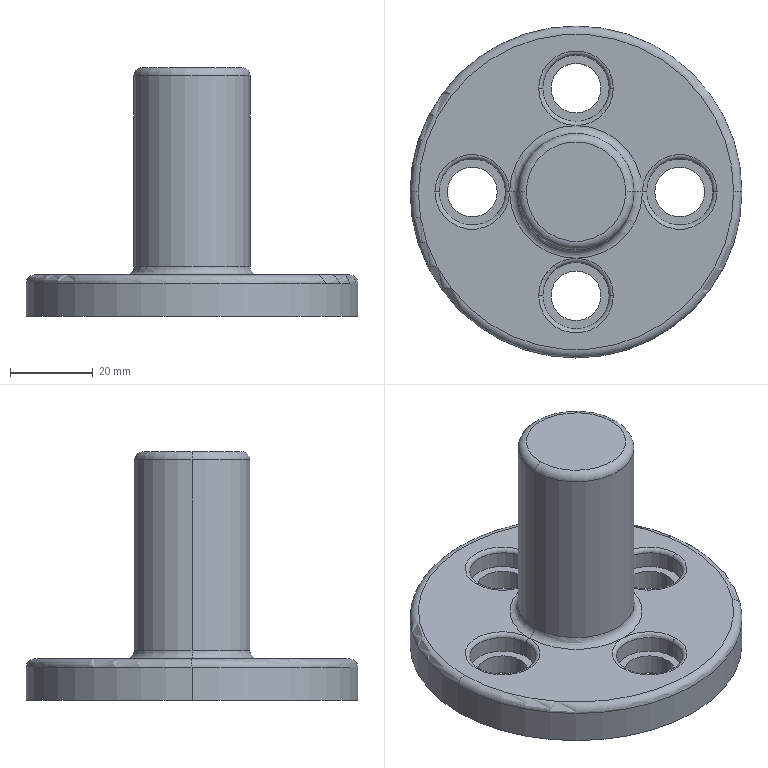Part | SolidWorks | features Fillet 4, ICE 3, Extrusion 1 | 1 solid | 41 faces | box 80 x 80 x 60 mm | volume 74517 mm3 | cylinder 20 | torus 14 | plane 7 | commonest cylinder face diameters 12 x8 16 x8 28 x2 80 x2
STEP:
#1=CARTESIAN_POINT('',(-14.,0.,12.));
#2=VERTEX_POINT('',#1);
#3=CARTESIAN_POINT('',(14.,0.,12.));
#4=VERTEX_POINT('',#3);
#5=CARTESIAN_POINT('',(0.,0.,12.));
#6=DIRECTION('',(0.,0.,1.));
#7=DIRECTION('',(1.,0.,0.));
#8=AXIS2_PLACEMENT_3D('',#5,#6,#7);
#9=CIRCLE('',#8,14.);
#10=EDGE_CURVE('',#2,#4,#9,.T.);
#11=ORIENTED_EDGE('',*,*,#10,.F.);
#12=CARTESIAN_POINT('',(-16.,0.,10.));
#13=VERTEX_POINT('',#12);
#14=CARTESIAN_POINT('',(-16.,0.,12.));
#15=DIRECTION('',(0.,1.,0.));
#16=DIRECTION('',(-1.,0.,0.));
#17=AXIS2_PLACEMENT_3D('',#14,#15,#16);
#18=CIRCLE('',#17,2.);
#19=EDGE_CURVE('',#2,#13,#18,.T.);
#20=ORIENTED_EDGE('',*,*,#19,.T.);
#21=CARTESIAN_POINT('',(0.,-16.,10.));
#22=VERTEX_POINT('',#21);
#23=CARTESIAN_POINT('',(0.,0.,10.));
#24=DIRECTION('',(0.,0.,-1.));
#25=DIRECTION('',(1.,0.,0.));
#26=AXIS2_PLACEMENT_3D('',#23,#24,#25);
#27=CIRCLE('',#26,16.);
#28=EDGE_CURVE('',#22,#13,#27,.T.);
#29=ORIENTED_EDGE('',*,*,#28,.F.);
#30=CARTESIAN_POINT('',(16.,0.,10.));
#31=VERTEX_POINT('',#30);
#32=CARTESIAN_POINT('',(0.,0.,10.));
#33=DIRECTION('',(0.,0.,-1.));
#34=DIRECTION('',(1.,0.,0.));
#35=AXIS2_PLACEMENT_3D('',#32,#33,#34);
#36=CIRCLE('',#35,16.);
#37=EDGE_CURVE('',#31,#22,#36,.T.);
#38=ORIENTED_EDGE('',*,*,#37,.F.);
#39=CARTESIAN_POINT('',(16.,0.,12.));
#40=DIRECTION('',(0.,-1.,0.));
#41=DIRECTION('',(0.,0.,-1.));
#42=AXIS2_PLACEMENT_3D('',#39,#40,#41);
#43=CIRCLE('',#42,2.);
#44=EDGE_CURVE('',#4,#31,#43,.T.);
#45=ORIENTED_EDGE('',*,*,#44,.F.);
#46=EDGE_LOOP('',(#11,#20,#29,#38,#45));
#47=FACE_OUTER_BOUND('',#46,.T.);
#48=CARTESIAN_POINT('',(0.,0.,12.));
#49=DIRECTION('',(0.,0.,1.));
#50=DIRECTION('',(1.,0.,0.));
#51=AXIS2_PLACEMENT_3D('',#48,#49,#50);
#52=TOROIDAL_SURFACE('',#51,16.,2.);
#53=ADVANCED_FACE('',(#47),#52,.F.);
#54=CARTESIAN_POINT('',(-14.,0.,58.));
#55=VERTEX_POINT('',#54);
#56=CARTESIAN_POINT('',(14.,0.,58.));
#57=VERTEX_POINT('',#56);
#58=CARTESIAN_POINT('',(0.,0.,58.));
#59=DIRECTION('',(0.,0.,-1.));
#60=DIRECTION('',(1.,0.,0.));
#61=AXIS2_PLACEMENT_3D('',#58,#59,#60);
#62=CIRCLE('',#61,14.);
#63=EDGE_CURVE('',#55,#57,#62,.T.);
#64=ORIENTED_EDGE('',*,*,#63,.F.);
#65=CARTESIAN_POINT('',(-12.,0.,60.));
#66=VERTEX_POINT('',#65);
#67=CARTESIAN_POINT('',(-12.,0.,58.));
#68=DIRECTION('',(0.,1.,0.));
#69=DIRECTION('',(-1.,0.,0.));
#70=AXIS2_PLACEMENT_3D('',#67,#68,#69);
#71=CIRCLE('',#70,2.);
#72=EDGE_CURVE('',#55,#66,#71,.T.);
#73=ORIENTED_EDGE('',*,*,#72,.T.);
#74=CARTESIAN_POINT('',(12.,0.,60.));
#75=VERTEX_POINT('',#74);
#76=CARTESIAN_POINT('',(0.,0.,60.));
#77=DIRECTION('',(0.,0.,1.));
#78=DIRECTION('',(1.,0.,0.));
#79=AXIS2_PLACEMENT_3D('',#76,#77,#78);
#80=CIRCLE('',#79,12.);
#81=EDGE_CURVE('',#75,#66,#80,.T.);
#82=ORIENTED_EDGE('',*,*,#81,.F.);
#83=CARTESIAN_POINT('',(12.,0.,58.));
#84=DIRECTION('',(0.,-1.,0.));
#85=DIRECTION('',(0.,0.,-1.));
#86=AXIS2_PLACEMENT_3D('',#83,#84,#85);
#87=CIRCLE('',#86,2.);
#88=EDGE_CURVE('',#57,#75,#87,.T.);
#89=ORIENTED_EDGE('',*,*,#88,.F.);
#90=EDGE_LOOP('',(#64,#73,#82,#89));
#91=FACE_OUTER_BOUND('',#90,.T.);
#92=CARTESIAN_POINT('',(0.,0.,58.));
#93=DIRECTION('',(0.,0.,1.));
#94=DIRECTION('',(1.,0.,0.));
#95=AXIS2_PLACEMENT_3D('',#92,#93,#94);
#96=TOROIDAL_SURFACE('',#95,12.,2.);
#97=ADVANCED_FACE('',(#91),#96,.T.);
#98=ORIENTED_EDGE('',*,*,#63,.T.);
#99=CARTESIAN_POINT('',(14.,0.,60.));
#100=DIRECTION('',(0.,0.,-1.));
#101=VECTOR('',#100,1000.);
#102=LINE('',#99,#101);
#103=EDGE_CURVE('',#57,#4,#102,.T.);
#104=ORIENTED_EDGE('',*,*,#103,.T.);
#105=CARTESIAN_POINT('',(0.,0.,12.));
#106=DIRECTION('',(0.,0.,1.));
#107=DIRECTION('',(1.,0.,0.));
#108=AXIS2_PLACEMENT_3D('',#105,#106,#107);
#109=CIRCLE('',#108,14.);
#110=EDGE_CURVE('',#4,#2,#109,.T.);
#111=ORIENTED_EDGE('',*,*,#110,.T.);
#112=CARTESIAN_POINT('',(-14.,0.,60.));
#113=DIRECTION('',(0.,0.,-1.));
#114=VECTOR('',#113,1000.);
#115=LINE('',#112,#114);
#116=EDGE_CURVE('',#55,#2,#115,.T.);
#117=ORIENTED_EDGE('',*,*,#116,.F.);
#118=EDGE_LOOP('',(#98,#104,#111,#117));
#119=FACE_OUTER_BOUND('',#118,.T.);
#120=CARTESIAN_POINT('',(0.,0.,60.));
#121=DIRECTION('',(0.,0.,-1.));
#122=DIRECTION('',(-1.,0.,0.));
#123=AXIS2_PLACEMENT_3D('',#120,#121,#122);
#124=CYLINDRICAL_SURFACE('',#123,14.);
#125=ADVANCED_FACE('',(#119),#124,.T.);
#126=CARTESIAN_POINT('',(-31.,0.,0.));
#127=VERTEX_POINT('',#126);
#128=CARTESIAN_POINT('',(-19.,0.,0.));
#129=VERTEX_POINT('',#128);
#130=CARTESIAN_POINT('',(-25.,0.,0.));
#131=DIRECTION('',(0.,0.,1.));
#132=DIRECTION('',(1.,0.,0.));
#133=AXIS2_PLACEMENT_3D('',#130,#131,#132);
#134=CIRCLE('',#133,6.);
#135=EDGE_CURVE('',#127,#129,#134,.T.);
#136=ORIENTED_EDGE('',*,*,#135,.F.);
#137=CARTESIAN_POINT('',(-31.,0.,5.));
#138=VERTEX_POINT('',#137);
#139=CARTESIAN_POINT('',(-31.,0.,0.));
#140=DIRECTION('',(0.,0.,1.));
#141=VECTOR('',#140,1000.);
#142=LINE('',#139,#141);
#143=EDGE_CURVE('',#127,#138,#142,.T.);
#144=ORIENTED_EDGE('',*,*,#143,.T.);
#145=CARTESIAN_POINT('',(-19.,0.,5.));
#146=VERTEX_POINT('',#145);
#147=CARTESIAN_POINT('',(-25.,0.,5.));
#148=DIRECTION('',(0.,0.,1.));
#149=DIRECTION('',(1.,0.,0.));
#150=AXIS2_PLACEMENT_3D('',#147,#148,#149);
#151=CIRCLE('',#150,6.);
#152=EDGE_CURVE('',#138,#146,#151,.T.);
#153=ORIENTED_EDGE('',*,*,#152,.T.);
#154=CARTESIAN_POINT('',(-19.,0.,0.));
#155=DIRECTION('',(0.,0.,1.));
#156=VECTOR('',#155,1000.);
#157=LINE('',#154,#156);
#158=EDGE_CURVE('',#129,#146,#157,.T.);
#159=ORIENTED_EDGE('',*,*,#158,.F.);
#160=EDGE_LOOP('',(#136,#144,#153,#159));
#161=FACE_OUTER_BOUND('',#160,.T.);
#162=CARTESIAN_POINT('',(-25.,0.,0.));
#163=DIRECTION('',(0.,0.,1.));
#164=DIRECTION('',(1.,0.,0.));
#165=AXIS2_PLACEMENT_3D('',#162,#163,#164);
#166=CYLINDRICAL_SURFACE('',#165,6.);
#167=ADVANCED_FACE('',(#161),#166,.F.);
#168=CARTESIAN_POINT('',(-6.,-25.,0.));
#169=VERTEX_POINT('',#168);
#170=CARTESIAN_POINT('',(6.,-25.,0.));
#171=VERTEX_POINT('',#170);
#172=CARTESIAN_POINT('',(0.,-25.,0.));
#173=DIRECTION('',(0.,0.,1.));
#174=DIRECTION('',(1.,0.,0.));
#175=AXIS2_PLACEMENT_3D('',#172,#173,#174);
#176=CIRCLE('',#175,6.);
#177=EDGE_CURVE('',#169,#171,#176,.T.);
#178=ORIENTED_EDGE('',*,*,#177,.F.);
#179=CARTESIAN_POINT('',(-6.,-25.,5.));
#180=VERTEX_POINT('',#179);
#181=CARTESIAN_POINT('',(-6.,-25.,0.));
#182=DIRECTION('',(0.,0.,1.));
#183=VECTOR('',#182,1000.);
#184=LINE('',#181,#183);
#185=EDGE_CURVE('',#169,#180,#184,.T.);
#186=ORIENTED_EDGE('',*,*,#185,.T.);
#187=CARTESIAN_POINT('',(6.,-25.,5.));
#188=VERTEX_POINT('',#187);
#189=CARTESIAN_POINT('',(0.,-25.,5.));
#190=DIRECTION('',(0.,0.,1.));
#191=DIRECTION('',(1.,0.,0.));
#192=AXIS2_PLACEMENT_3D('',#189,#190,#191);
#193=CIRCLE('',#192,6.);
#194=EDGE_CURVE('',#180,#188,#193,.T.);
#195=ORIENTED_EDGE('',*,*,#194,.T.);
#196=CARTESIAN_POINT('',(6.,-25.,0.));
#197=DIRECTION('',(0.,0.,1.));
#198=VECTOR('',#197,1000.);
#199=LINE('',#196,#198);
#200=EDGE_CURVE('',#171,#188,#199,.T.);
#201=ORIENTED_EDGE('',*,*,#200,.F.);
#202=EDGE_LOOP('',(#178,#186,#195,#201));
#203=FACE_OUTER_BOUND('',#202,.T.);
#204=CARTESIAN_POINT('',(0.,-25.,0.));
#205=DIRECTION('',(0.,0.,1.));
#206=DIRECTION('',(1.,0.,0.));
#207=AXIS2_PLACEMENT_3D('',#204,#205,#206);
#208=CYLINDRICAL_SURFACE('',#207,6.);
#209=ADVANCED_FACE('',(#203),#208,.F.);
#210=CARTESIAN_POINT('',(19.,0.,0.));
#211=VERTEX_POINT('',#210);
#212=CARTESIAN_POINT('',(31.,0.,0.));
#213=VERTEX_POINT('',#212);
#214=CARTESIAN_POINT('',(25.,0.,0.));
#215=DIRECTION('',(0.,0.,1.));
#216=DIRECTION('',(1.,0.,0.));
#217=AXIS2_PLACEMENT_3D('',#214,#215,#216);
#218=CIRCLE('',#217,6.);
#219=EDGE_CURVE('',#211,#213,#218,.T.);
#220=ORIENTED_EDGE('',*,*,#219,.F.);
#221=CARTESIAN_POINT('',(19.,0.,5.));
#222=VERTEX_POINT('',#221);
#223=CARTESIAN_POINT('',(19.,0.,0.));
#224=DIRECTION('',(0.,0.,1.));
#225=VECTOR('',#224,1000.);
#226=LINE('',#223,#225);
#227=EDGE_CURVE('',#211,#222,#226,.T.);
#228=ORIENTED_EDGE('',*,*,#227,.T.);
#229=CARTESIAN_POINT('',(31.,0.,5.));
#230=VERTEX_POINT('',#229);
#231=CARTESIAN_POINT('',(25.,0.,5.));
#232=DIRECTION('',(0.,0.,1.));
#233=DIRECTION('',(1.,0.,0.));
#234=AXIS2_PLACEMENT_3D('',#231,#232,#233);
#235=CIRCLE('',#234,6.);
#236=EDGE_CURVE('',#222,#230,#235,.T.);
#237=ORIENTED_EDGE('',*,*,#236,.T.);
#238=CARTESIAN_POINT('',(31.,0.,0.));
#239=DIRECTION('',(0.,0.,1.));
#240=VECTOR('',#239,1000.);
#241=LINE('',#238,#240);
#242=EDGE_CURVE('',#213,#230,#241,.T.);
#243=ORIENTED_EDGE('',*,*,#242,.F.);
#244=EDGE_LOOP('',(#220,#228,#237,#243));
#245=FACE_OUTER_BOUND('',#244,.T.);
#246=CARTESIAN_POINT('',(25.,0.,0.));
#247=DIRECTION('',(0.,0.,1.));
#248=DIRECTION('',(1.,0.,0.));
#249=AXIS2_PLACEMENT_3D('',#246,#247,#248);
#250=CYLINDRICAL_SURFACE('',#249,6.);
#251=ADVANCED_FACE('',(#245),#250,.F.);
#252=CARTESIAN_POINT('',(-6.,25.,0.));
#253=VERTEX_POINT('',#252);
#254=CARTESIAN_POINT('',(6.,25.,0.));
#255=VERTEX_POINT('',#254);
#256=CARTESIAN_POINT('',(0.,25.,0.));
#257=DIRECTION('',(0.,0.,1.));
#258=DIRECTION('',(1.,0.,0.));
#259=AXIS2_PLACEMENT_3D('',#256,#257,#258);
#260=CIRCLE('',#259,6.);
#261=EDGE_CURVE('',#253,#255,#260,.T.);
#262=ORIENTED_EDGE('',*,*,#261,.F.);
#263=CARTESIAN_POINT('',(-6.,25.,5.));
#264=VERTEX_POINT('',#263);
#265=CARTESIAN_POINT('',(-6.,25.,0.));
#266=DIRECTION('',(0.,0.,1.));
#267=VECTOR('',#266,1000.);
#268=LINE('',#265,#267);
#269=EDGE_CURVE('',#253,#264,#268,.T.);
#270=ORIENTED_EDGE('',*,*,#269,.T.);
#271=CARTESIAN_POINT('',(6.,25.,5.));
#272=VERTEX_POINT('',#271);
#273=CARTESIAN_POINT('',(0.,25.,5.));
#274=DIRECTION('',(0.,0.,1.));
#275=DIRECTION('',(1.,0.,0.));
#276=AXIS2_PLACEMENT_3D('',#273,#274,#275);
#277=CIRCLE('',#276,6.);
#278=EDGE_CURVE('',#264,#272,#277,.T.);
#279=ORIENTED_EDGE('',*,*,#278,.T.);
#280=CARTESIAN_POINT('',(6.,25.,0.));
#281=DIRECTION('',(0.,0.,1.));
#282=VECTOR('',#281,1000.);
#283=LINE('',#280,#282);
#284=EDGE_CURVE('',#255,#272,#283,.T.);
#285=ORIENTED_EDGE('',*,*,#284,.F.);
#286=EDGE_LOOP('',(#262,#270,#279,#285));
#287=FACE_OUTER_BOUND('',#286,.T.);
#288=CARTESIAN_POINT('',(0.,25.,0.));
#289=DIRECTION('',(0.,0.,1.));
#290=DIRECTION('',(1.,0.,0.));
#291=AXIS2_PLACEMENT_3D('',#288,#289,#290);
#292=CYLINDRICAL_SURFACE('',#291,6.);
#293=ADVANCED_FACE('',(#287),#292,.F.);
#294=CARTESIAN_POINT('',(-34.,0.,10.));
#295=VERTEX_POINT('',#294);
#296=CARTESIAN_POINT('',(-25.,0.,10.));
#297=DIRECTION('',(0.,0.,-1.));
#298=DIRECTION('',(1.,0.,0.));
#299=AXIS2_PLACEMENT_3D('',#296,#297,#298);
#300=CIRCLE('',#299,9.);
#301=EDGE_CURVE('',#295,#13,#300,.T.);
#302=ORIENTED_EDGE('',*,*,#301,.F.);
#303=CARTESIAN_POINT('',(-33.,0.,9.));
#304=VERTEX_POINT('',#303);
#305=CARTESIAN_POINT('',(-34.,0.,9.));
#306=DIRECTION('',(0.,1.,0.));
#307=DIRECTION('',(-1.,0.,0.));
#308=AXIS2_PLACEMENT_3D('',#305,#306,#307);
#309=CIRCLE('',#308,1.);
#310=EDGE_CURVE('',#295,#304,#309,.T.);
#311=ORIENTED_EDGE('',*,*,#310,.T.);
#312=CARTESIAN_POINT('',(-17.,0.,9.));
#313=VERTEX_POINT('',#312);
#314=CARTESIAN_POINT('',(-25.,0.,9.));
#315=DIRECTION('',(0.,0.,1.));
#316=DIRECTION('',(1.,0.,0.));
#317=AXIS2_PLACEMENT_3D('',#314,#315,#316);
#318=CIRCLE('',#317,8.);
#319=EDGE_CURVE('',#313,#304,#318,.T.);
#320=ORIENTED_EDGE('',*,*,#319,.F.);
#321=CARTESIAN_POINT('',(-16.,0.,9.));
#322=DIRECTION('',(0.,-1.,0.));
#323=DIRECTION('',(0.,0.,-1.));
#324=AXIS2_PLACEMENT_3D('',#321,#322,#323);
#325=CIRCLE('',#324,1.);
#326=EDGE_CURVE('',#13,#313,#325,.T.);
#327=ORIENTED_EDGE('',*,*,#326,.F.);
#328=EDGE_LOOP('',(#302,#311,#320,#327));
#329=FACE_OUTER_BOUND('',#328,.T.);
#330=CARTESIAN_POINT('',(-25.,0.,9.));
#331=DIRECTION('',(0.,0.,1.));
#332=DIRECTION('',(1.,0.,0.));
#333=AXIS2_PLACEMENT_3D('',#330,#331,#332);
#334=TOROIDAL_SURFACE('',#333,9.,1.);
#335=ADVANCED_FACE('',(#329),#334,.T.);
#336=CARTESIAN_POINT('',(-9.,25.,10.));
#337=VERTEX_POINT('',#336);
#338=CARTESIAN_POINT('',(9.,25.,10.));
#339=VERTEX_POINT('',#338);
#340=CARTESIAN_POINT('',(0.,25.,10.));
#341=DIRECTION('',(0.,0.,-1.));
#342=DIRECTION('',(1.,0.,0.));
#343=AXIS2_PLACEMENT_3D('',#340,#341,#342);
#344=CIRCLE('',#343,9.);
#345=EDGE_CURVE('',#337,#339,#344,.T.);
#346=ORIENTED_EDGE('',*,*,#345,.F.);
#347=CARTESIAN_POINT('',(-8.,25.,9.));
#348=VERTEX_POINT('',#347);
#349=CARTESIAN_POINT('',(-9.,25.,9.));
#350=DIRECTION('',(0.,1.,0.));
#351=DIRECTION('',(-1.,0.,0.));
#352=AXIS2_PLACEMENT_3D('',#349,#350,#351);
#353=CIRCLE('',#352,1.);
#354=EDGE_CURVE('',#337,#348,#353,.T.);
#355=ORIENTED_EDGE('',*,*,#354,.T.);
#356=CARTESIAN_POINT('',(8.,25.,9.));
#357=VERTEX_POINT('',#356);
#358=CARTESIAN_POINT('',(0.,25.,9.));
#359=DIRECTION('',(0.,0.,1.));
#360=DIRECTION('',(1.,0.,0.));
#361=AXIS2_PLACEMENT_3D('',#358,#359,#360);
#362=CIRCLE('',#361,8.);
#363=EDGE_CURVE('',#357,#348,#362,.T.);
#364=ORIENTED_EDGE('',*,*,#363,.F.);
#365=CARTESIAN_POINT('',(9.,25.,9.));
#366=DIRECTION('',(0.,-1.,0.));
#367=DIRECTION('',(0.,0.,-1.));
#368=AXIS2_PLACEMENT_3D('',#365,#366,#367);
#369=CIRCLE('',#368,1.);
#370=EDGE_CURVE('',#339,#357,#369,.T.);
#371=ORIENTED_EDGE('',*,*,#370,.F.);
#372=EDGE_LOOP('',(#346,#355,#364,#371));
#373=FACE_OUTER_BOUND('',#372,.T.);
#374=CARTESIAN_POINT('',(0.,25.,9.));
#375=DIRECTION('',(0.,0.,1.));
#376=DIRECTION('',(1.,0.,0.));
#377=AXIS2_PLACEMENT_3D('',#374,#375,#376);
#378=TOROIDAL_SURFACE('',#377,9.,1.);
#379=ADVANCED_FACE('',(#373),#378,.T.);
#380=CARTESIAN_POINT('',(34.,0.,10.));
#381=VERTEX_POINT('',#380);
#382=CARTESIAN_POINT('',(25.,0.,10.));
#383=DIRECTION('',(0.,0.,-1.));
#384=DIRECTION('',(1.,0.,0.));
#385=AXIS2_PLACEMENT_3D('',#382,#383,#384);
#386=CIRCLE('',#385,9.);
#387=EDGE_CURVE('',#31,#381,#386,.T.);
#388=ORIENTED_EDGE('',*,*,#387,.F.);
#389=CARTESIAN_POINT('',(17.,0.,9.));
#390=VERTEX_POINT('',#389);
#391=CARTESIAN_POINT('',(16.,0.,9.));
#392=DIRECTION('',(0.,1.,0.));
#393=DIRECTION('',(-1.,0.,0.));
#394=AXIS2_PLACEMENT_3D('',#391,#392,#393);
#395=CIRCLE('',#394,1.);
#396=EDGE_CURVE('',#31,#390,#395,.T.);
#397=ORIENTED_EDGE('',*,*,#396,.T.);
#398=CARTESIAN_POINT('',(33.,0.,9.));
#399=VERTEX_POINT('',#398);
#400=CARTESIAN_POINT('',(25.,0.,9.));
#401=DIRECTION('',(0.,0.,1.));
#402=DIRECTION('',(1.,0.,0.));
#403=AXIS2_PLACEMENT_3D('',#400,#401,#402);
#404=CIRCLE('',#403,8.);
#405=EDGE_CURVE('',#399,#390,#404,.T.);
#406=ORIENTED_EDGE('',*,*,#405,.F.);
#407=CARTESIAN_POINT('',(34.,0.,9.));
#408=DIRECTION('',(0.,-1.,0.));
#409=DIRECTION('',(0.,0.,-1.));
#410=AXIS2_PLACEMENT_3D('',#407,#408,#409);
#411=CIRCLE('',#410,1.);
#412=EDGE_CURVE('',#381,#399,#411,.T.);
#413=ORIENTED_EDGE('',*,*,#412,.F.);
#414=EDGE_LOOP('',(#388,#397,#406,#413));
#415=FACE_OUTER_BOUND('',#414,.T.);
#416=CARTESIAN_POINT('',(25.,0.,9.));
#417=DIRECTION('',(0.,0.,1.));
#418=DIRECTION('',(1.,0.,0.));
#419=AXIS2_PLACEMENT_3D('',#416,#417,#418);
#420=TOROIDAL_SURFACE('',#419,9.,1.);
#421=ADVANCED_FACE('',(#415),#420,.T.);
#422=CARTESIAN_POINT('',(-9.,-25.,10.));
#423=VERTEX_POINT('',#422);
#424=CARTESIAN_POINT('',(0.,-25.,10.));
#425=DIRECTION('',(0.,0.,-1.));
#426=DIRECTION('',(1.,0.,0.));
#427=AXIS2_PLACEMENT_3D('',#424,#425,#426);
#428=CIRCLE('',#427,9.);
#429=EDGE_CURVE('',#423,#22,#428,.T.);
#430=ORIENTED_EDGE('',*,*,#429,.F.);
#431=CARTESIAN_POINT('',(-8.,-25.,9.));
#432=VERTEX_POINT('',#431);
#433=CARTESIAN_POINT('',(-9.,-25.,9.));
#434=DIRECTION('',(0.,1.,0.));
#435=DIRECTION('',(-1.,0.,0.));
#436=AXIS2_PLACEMENT_3D('',#433,#434,#435);
#437=CIRCLE('',#436,1.);
#438=EDGE_CURVE('',#423,#432,#437,.T.);
#439=ORIENTED_EDGE('',*,*,#438,.T.);
#440=CARTESIAN_POINT('',(8.,-25.,9.));
#441=VERTEX_POINT('',#440);
#442=CARTESIAN_POINT('',(0.,-25.,9.));
#443=DIRECTION('',(0.,0.,1.));
#444=DIRECTION('',(1.,0.,0.));
#445=AXIS2_PLACEMENT_3D('',#442,#443,#444);
#446=CIRCLE('',#445,8.);
#447=EDGE_CURVE('',#441,#432,#446,.T.);
#448=ORIENTED_EDGE('',*,*,#447,.F.);
#449=CARTESIAN_POINT('',(9.,-25.,10.));
#450=VERTEX_POINT('',#449);
#451=CARTESIAN_POINT('',(9.,-25.,9.));
#452=DIRECTION('',(0.,-1.,0.));
#453=DIRECTION('',(0.,0.,-1.));
#454=AXIS2_PLACEMENT_3D('',#451,#452,#453);
#455=CIRCLE('',#454,1.);
#456=EDGE_CURVE('',#450,#441,#455,.T.);
#457=ORIENTED_EDGE('',*,*,#456,.F.);
#458=CARTESIAN_POINT('',(0.,-25.,10.));
#459=DIRECTION('',(0.,0.,-1.));
#460=DIRECTION('',(1.,0.,0.));
#461=AXIS2_PLACEMENT_3D('',#458,#459,#460);
#462=CIRCLE('',#461,9.);
#463=EDGE_CURVE('',#22,#450,#462,.T.);
#464=ORIENTED_EDGE('',*,*,#463,.F.);
#465=EDGE_LOOP('',(#430,#439,#448,#457,#464));
#466=FACE_OUTER_BOUND('',#465,.T.);
#467=CARTESIAN_POINT('',(0.,-25.,9.));
#468=DIRECTION('',(0.,0.,1.));
#469=DIRECTION('',(1.,0.,0.));
#470=AXIS2_PLACEMENT_3D('',#467,#468,#469);
#471=TOROIDAL_SURFACE('',#470,9.,1.);
#472=ADVANCED_FACE('',(#466),#471,.T.);
#473=CARTESIAN_POINT('',(-8.,25.,5.));
#474=VERTEX_POINT('',#473);
#475=CARTESIAN_POINT('',(8.,25.,5.));
#476=VERTEX_POINT('',#475);
#477=CARTESIAN_POINT('',(0.,25.,5.));
#478=DIRECTION('',(0.,0.,1.));
#479=DIRECTION('',(1.,0.,0.));
#480=AXIS2_PLACEMENT_3D('',#477,#478,#479);
#481=CIRCLE('',#480,8.);
#482=EDGE_CURVE('',#474,#476,#481,.T.);
#483=ORIENTED_EDGE('',*,*,#482,.F.);
#484=CARTESIAN_POINT('',(-8.,25.,5.));
#485=DIRECTION('',(0.,0.,1.));
#486=VECTOR('',#485,1000.);
#487=LINE('',#484,#486);
#488=EDGE_CURVE('',#474,#348,#487,.T.);
#489=ORIENTED_EDGE('',*,*,#488,.T.);
#490=CARTESIAN_POINT('',(0.,25.,9.));
#491=DIRECTION('',(0.,0.,1.));
#492=DIRECTION('',(1.,0.,0.));
#493=AXIS2_PLACEMENT_3D('',#490,#491,#492);
#494=CIRCLE('',#493,8.);
#495=EDGE_CURVE('',#348,#357,#494,.T.);
#496=ORIENTED_EDGE('',*,*,#495,.T.);
#497=CARTESIAN_POINT('',(8.,25.,5.));
#498=DIRECTION('',(0.,0.,1.));
#499=VECTOR('',#498,1000.);
#500=LINE('',#497,#499);
#501=EDGE_CURVE('',#476,#357,#500,.T.);
#502=ORIENTED_EDGE('',*,*,#501,.F.);
#503=EDGE_LOOP('',(#483,#489,#496,#502));
#504=FACE_OUTER_BOUND('',#503,.T.);
#505=CARTESIAN_POINT('',(0.,25.,5.));
#506=DIRECTION('',(0.,0.,1.));
#507=DIRECTION('',(1.,0.,0.));
#508=AXIS2_PLACEMENT_3D('',#505,#506,#507);
#509=CYLINDRICAL_SURFACE('',#508,8.);
#510=ADVANCED_FACE('',(#504),#509,.F.);
#511=CARTESIAN_POINT('',(17.,0.,5.));
#512=VERTEX_POINT('',#511);
#513=CARTESIAN_POINT('',(33.,0.,5.));
#514=VERTEX_POINT('',#513);
#515=CARTESIAN_POINT('',(25.,0.,5.));
#516=DIRECTION('',(0.,0.,1.));
#517=DIRECTION('',(1.,0.,0.));
#518=AXIS2_PLACEMENT_3D('',#515,#516,#517);
#519=CIRCLE('',#518,8.);
#520=EDGE_CURVE('',#512,#514,#519,.T.);
#521=ORIENTED_EDGE('',*,*,#520,.F.);
#522=CARTESIAN_POINT('',(17.,0.,5.));
#523=DIRECTION('',(0.,0.,1.));
#524=VECTOR('',#523,1000.);
#525=LINE('',#522,#524);
#526=EDGE_CURVE('',#512,#390,#525,.T.);
#527=ORIENTED_EDGE('',*,*,#526,.T.);
#528=CARTESIAN_POINT('',(25.,0.,9.));
#529=DIRECTION('',(0.,0.,1.));
#530=DIRECTION('',(1.,0.,0.));
#531=AXIS2_PLACEMENT_3D('',#528,#529,#530);
#532=CIRCLE('',#531,8.);
#533=EDGE_CURVE('',#390,#399,#532,.T.);
#534=ORIENTED_EDGE('',*,*,#533,.T.);
#535=CARTESIAN_POINT('',(33.,0.,5.));
#536=DIRECTION('',(0.,0.,1.));
#537=VECTOR('',#536,1000.);
#538=LINE('',#535,#537);
#539=EDGE_CURVE('',#514,#399,#538,.T.);
#540=ORIENTED_EDGE('',*,*,#539,.F.);
#541=EDGE_LOOP('',(#521,#527,#534,#540));
#542=FACE_OUTER_BOUND('',#541,.T.);
#543=CARTESIAN_POINT('',(25.,0.,5.));
#544=DIRECTION('',(0.,0.,1.));
#545=DIRECTION('',(1.,0.,0.));
#546=AXIS2_PLACEMENT_3D('',#543,#544,#545);
#547=CYLINDRICAL_SURFACE('',#546,8.);
#548=ADVANCED_FACE('',(#542),#547,.F.);
#549=CARTESIAN_POINT('',(-8.,-25.,5.));
#550=VERTEX_POINT('',#549);
#551=CARTESIAN_POINT('',(8.,-25.,5.));
#552=VERTEX_POINT('',#551);
#553=CARTESIAN_POINT('',(0.,-25.,5.));
#554=DIRECTION('',(0.,0.,1.));
#555=DIRECTION('',(1.,0.,0.));
#556=AXIS2_PLACEMENT_3D('',#553,#554,#555);
#557=CIRCLE('',#556,8.);
#558=EDGE_CURVE('',#550,#552,#557,.T.);
#559=ORIENTED_EDGE('',*,*,#558,.F.);
#560=CARTESIAN_POINT('',(-8.,-25.,5.));
#561=DIRECTION('',(0.,0.,1.));
#562=VECTOR('',#561,1000.);
#563=LINE('',#560,#562);
#564=EDGE_CURVE('',#550,#432,#563,.T.);
#565=ORIENTED_EDGE('',*,*,#564,.T.);
#566=CARTESIAN_POINT('',(0.,-25.,9.));
#567=DIRECTION('',(0.,0.,1.));
#568=DIRECTION('',(1.,0.,0.));
#569=AXIS2_PLACEMENT_3D('',#566,#567,#568);
#570=CIRCLE('',#569,8.);
#571=EDGE_CURVE('',#432,#441,#570,.T.);
#572=ORIENTED_EDGE('',*,*,#571,.T.);
#573=CARTESIAN_POINT('',(8.,-25.,5.));
#574=DIRECTION('',(0.,0.,1.));
#575=VECTOR('',#574,1000.);
#576=LINE('',#573,#575);
#577=EDGE_CURVE('',#552,#441,#576,.T.);
#578=ORIENTED_EDGE('',*,*,#577,.F.);
#579=EDGE_LOOP('',(#559,#565,#572,#578));
#580=FACE_OUTER_BOUND('',#579,.T.);
#581=CARTESIAN_POINT('',(0.,-25.,5.));
#582=DIRECTION('',(0.,0.,1.));
#583=DIRECTION('',(1.,0.,0.));
#584=AXIS2_PLACEMENT_3D('',#581,#582,#583);
#585=CYLINDRICAL_SURFACE('',#584,8.);
#586=ADVANCED_FACE('',(#580),#585,.F.);
#587=CARTESIAN_POINT('',(-33.,0.,5.));
#588=VERTEX_POINT('',#587);
#589=CARTESIAN_POINT('',(-17.,0.,5.));
#590=VERTEX_POINT('',#589);
#591=CARTESIAN_POINT('',(-25.,0.,5.));
#592=DIRECTION('',(0.,0.,1.));
#593=DIRECTION('',(1.,0.,0.));
#594=AXIS2_PLACEMENT_3D('',#591,#592,#593);
#595=CIRCLE('',#594,8.);
#596=EDGE_CURVE('',#588,#590,#595,.T.);
#597=ORIENTED_EDGE('',*,*,#596,.F.);
#598=CARTESIAN_POINT('',(-33.,0.,5.));
#599=DIRECTION('',(0.,0.,1.));
#600=VECTOR('',#599,1000.);
#601=LINE('',#598,#600);
#602=EDGE_CURVE('',#588,#304,#601,.T.);
#603=ORIENTED_EDGE('',*,*,#602,.T.);
#604=CARTESIAN_POINT('',(-25.,0.,9.));
#605=DIRECTION('',(0.,0.,1.));
#606=DIRECTION('',(1.,0.,0.));
#607=AXIS2_PLACEMENT_3D('',#604,#605,#606);
#608=CIRCLE('',#607,8.);
#609=EDGE_CURVE('',#304,#313,#608,.T.);
#610=ORIENTED_EDGE('',*,*,#609,.T.);
#611=CARTESIAN_POINT('',(-17.,0.,5.));
#612=DIRECTION('',(0.,0.,1.));
#613=VECTOR('',#612,1000.);
#614=LINE('',#611,#613);
#615=EDGE_CURVE('',#590,#313,#614,.T.);
#616=ORIENTED_EDGE('',*,*,#615,.F.);
#617=EDGE_LOOP('',(#597,#603,#610,#616));
#618=FACE_OUTER_BOUND('',#617,.T.);
#619=CARTESIAN_POINT('',(-25.,0.,5.));
#620=DIRECTION('',(0.,0.,1.));
#621=DIRECTION('',(1.,0.,0.));
#622=AXIS2_PLACEMENT_3D('',#619,#620,#621);
#623=CYLINDRICAL_SURFACE('',#622,8.);
#624=ADVANCED_FACE('',(#618),#623,.F.);
#625=CARTESIAN_POINT('',(-40.,0.,8.));
#626=VERTEX_POINT('',#625);
#627=CARTESIAN_POINT('',(40.,0.,8.));
#628=VERTEX_POINT('',#627);
#629=CARTESIAN_POINT('',(0.,0.,8.));
#630=DIRECTION('',(0.,0.,-1.));
#631=DIRECTION('',(1.,0.,0.));
#632=AXIS2_PLACEMENT_3D('',#629,#630,#631);
#633=CIRCLE('',#632,40.);
#634=EDGE_CURVE('',#626,#628,#633,.T.);
#635=ORIENTED_EDGE('',*,*,#634,.F.);
#636=CARTESIAN_POINT('',(-38.,0.,10.));
#637=VERTEX_POINT('',#636);
#638=CARTESIAN_POINT('',(-38.,0.,8.));
#639=DIRECTION('',(0.,1.,0.));
#640=DIRECTION('',(-1.,0.,0.));
#641=AXIS2_PLACEMENT_3D('',#638,#639,#640);
#642=CIRCLE('',#641,2.);
#643=EDGE_CURVE('',#626,#637,#642,.T.);
#644=ORIENTED_EDGE('',*,*,#643,.T.);
#645=CARTESIAN_POINT('',(38.,0.,10.));
#646=VERTEX_POINT('',#645);
#647=CARTESIAN_POINT('',(0.,0.,10.));
#648=DIRECTION('',(0.,0.,1.));
#649=DIRECTION('',(1.,0.,0.));
#650=AXIS2_PLACEMENT_3D('',#647,#648,#649);
#651=CIRCLE('',#650,38.);
#652=EDGE_CURVE('',#646,#637,#651,.T.);
#653=ORIENTED_EDGE('',*,*,#652,.F.);
#654=CARTESIAN_POINT('',(38.,0.,8.));
#655=DIRECTION('',(0.,-1.,0.));
#656=DIRECTION('',(0.,0.,-1.));
#657=AXIS2_PLACEMENT_3D('',#654,#655,#656);
#658=CIRCLE('',#657,2.);
#659=EDGE_CURVE('',#628,#646,#658,.T.);
#660=ORIENTED_EDGE('',*,*,#659,.F.);
#661=EDGE_LOOP('',(#635,#644,#653,#660));
#662=FACE_OUTER_BOUND('',#661,.T.);
#663=CARTESIAN_POINT('',(0.,0.,8.));
#664=DIRECTION('',(0.,0.,1.));
#665=DIRECTION('',(1.,0.,0.));
#666=AXIS2_PLACEMENT_3D('',#663,#664,#665);
#667=TOROIDAL_SURFACE('',#666,38.,2.);
#668=ADVANCED_FACE('',(#662),#667,.T.);
#669=ORIENTED_EDGE('',*,*,#634,.T.);
#670=CARTESIAN_POINT('',(40.,0.,0.));
#671=VERTEX_POINT('',#670);
#672=CARTESIAN_POINT('',(40.,0.,10.));
#673=DIRECTION('',(0.,0.,-1.));
#674=VECTOR('',#673,1000.);
#675=LINE('',#672,#674);
#676=EDGE_CURVE('',#628,#671,#675,.T.);
#677=ORIENTED_EDGE('',*,*,#676,.T.);
#678=CARTESIAN_POINT('',(-40.,0.,0.));
#679=VERTEX_POINT('',#678);
#680=CARTESIAN_POINT('',(0.,0.,0.));
#681=DIRECTION('',(0.,0.,1.));
#682=DIRECTION('',(1.,0.,0.));
#683=AXIS2_PLACEMENT_3D('',#680,#681,#682);
#684=CIRCLE('',#683,40.);
#685=EDGE_CURVE('',#671,#679,#684,.T.);
#686=ORIENTED_EDGE('',*,*,#685,.T.);
#687=CARTESIAN_POINT('',(-40.,0.,10.));
#688=DIRECTION('',(0.,0.,-1.));
#689=VECTOR('',#688,1000.);
#690=LINE('',#687,#689);
#691=EDGE_CURVE('',#626,#679,#690,.T.);
#692=ORIENTED_EDGE('',*,*,#691,.F.);
#693=EDGE_LOOP('',(#669,#677,#686,#692));
#694=FACE_OUTER_BOUND('',#693,.T.);
#695=CARTESIAN_POINT('',(0.,0.,10.));
#696=DIRECTION('',(0.,0.,-1.));
#697=DIRECTION('',(-1.,0.,0.));
#698=AXIS2_PLACEMENT_3D('',#695,#696,#697);
#699=CYLINDRICAL_SURFACE('',#698,40.);
#700=ADVANCED_FACE('',(#694),#699,.T.);
#701=ORIENTED_EDGE('',*,*,#676,.F.);
#702=CARTESIAN_POINT('',(0.,0.,8.));
#703=DIRECTION('',(0.,0.,-1.));
#704=DIRECTION('',(1.,0.,0.));
#705=AXIS2_PLACEMENT_3D('',#702,#703,#704);
#706=CIRCLE('',#705,40.);
#707=EDGE_CURVE('',#628,#626,#706,.T.);
#708=ORIENTED_EDGE('',*,*,#707,.T.);
#709=ORIENTED_EDGE('',*,*,#691,.T.);
#710=CARTESIAN_POINT('',(0.,0.,0.));
#711=DIRECTION('',(0.,0.,1.));
#712=DIRECTION('',(1.,0.,0.));
#713=AXIS2_PLACEMENT_3D('',#710,#711,#712);
#714=CIRCLE('',#713,40.);
#715=EDGE_CURVE('',#679,#671,#714,.T.);
#716=ORIENTED_EDGE('',*,*,#715,.T.);
#717=EDGE_LOOP('',(#701,#708,#709,#716));
#718=FACE_OUTER_BOUND('',#717,.T.);
#719=CARTESIAN_POINT('',(0.,0.,10.));
#720=DIRECTION('',(0.,0.,-1.));
#721=DIRECTION('',(-1.,0.,0.));
#722=AXIS2_PLACEMENT_3D('',#719,#720,#721);
#723=CYLINDRICAL_SURFACE('',#722,40.);
#724=ADVANCED_FACE('',(#718),#723,.T.);
#725=ORIENTED_EDGE('',*,*,#387,.T.);
#726=CARTESIAN_POINT('',(25.,0.,10.));
#727=DIRECTION('',(0.,0.,-1.));
#728=DIRECTION('',(1.,0.,0.));
#729=AXIS2_PLACEMENT_3D('',#726,#727,#728);
#730=CIRCLE('',#729,9.);
#731=EDGE_CURVE('',#381,#31,#730,.T.);
#732=ORIENTED_EDGE('',*,*,#731,.T.);
#733=ORIENTED_EDGE('',*,*,#37,.T.);
#734=ORIENTED_EDGE('',*,*,#463,.T.);
#735=CARTESIAN_POINT('',(0.,-25.,10.));
#736=DIRECTION('',(0.,0.,-1.));
#737=DIRECTION('',(1.,0.,0.));
#738=AXIS2_PLACEMENT_3D('',#735,#736,#737);
#739=CIRCLE('',#738,9.);
#740=EDGE_CURVE('',#450,#423,#739,.T.);
#741=ORIENTED_EDGE('',*,*,#740,.T.);
#742=ORIENTED_EDGE('',*,*,#429,.T.);
#743=ORIENTED_EDGE('',*,*,#28,.T.);
#744=CARTESIAN_POINT('',(-25.,0.,10.));
#745=DIRECTION('',(0.,0.,-1.));
#746=DIRECTION('',(1.,0.,0.));
#747=AXIS2_PLACEMENT_3D('',#744,#745,#746);
#748=CIRCLE('',#747,9.);
#749=EDGE_CURVE('',#13,#295,#748,.T.);
#750=ORIENTED_EDGE('',*,*,#749,.T.);
#751=ORIENTED_EDGE('',*,*,#301,.T.);
#752=CARTESIAN_POINT('',(0.,16.,10.));
#753=VERTEX_POINT('',#752);
#754=CARTESIAN_POINT('',(0.,0.,10.));
#755=DIRECTION('',(0.,0.,-1.));
#756=DIRECTION('',(1.,0.,0.));
#757=AXIS2_PLACEMENT_3D('',#754,#755,#756);
#758=CIRCLE('',#757,16.);
#759=EDGE_CURVE('',#13,#753,#758,.T.);
#760=ORIENTED_EDGE('',*,*,#759,.T.);
#761=CARTESIAN_POINT('',(0.,25.,10.));
#762=DIRECTION('',(0.,0.,-1.));
#763=DIRECTION('',(1.,0.,0.));
#764=AXIS2_PLACEMENT_3D('',#761,#762,#763);
#765=CIRCLE('',#764,9.);
#766=EDGE_CURVE('',#753,#337,#765,.T.);
#767=ORIENTED_EDGE('',*,*,#766,.T.);
#768=ORIENTED_EDGE('',*,*,#345,.T.);
#769=CARTESIAN_POINT('',(0.,25.,10.));
#770=DIRECTION('',(0.,0.,-1.));
#771=DIRECTION('',(1.,0.,0.));
#772=AXIS2_PLACEMENT_3D('',#769,#770,#771);
#773=CIRCLE('',#772,9.);
#774=EDGE_CURVE('',#339,#753,#773,.T.);
#775=ORIENTED_EDGE('',*,*,#774,.T.);
#776=CARTESIAN_POINT('',(0.,0.,10.));
#777=DIRECTION('',(0.,0.,-1.));
#778=DIRECTION('',(1.,0.,0.));
#779=AXIS2_PLACEMENT_3D('',#776,#777,#778);
#780=CIRCLE('',#779,16.);
#781=EDGE_CURVE('',#753,#31,#780,.T.);
#782=ORIENTED_EDGE('',*,*,#781,.T.);
#783=EDGE_LOOP('',(#725,#732,#733,#734,#741,#742,#743,#750,#751,#760,#767,#768,#775,#782));
#784=FACE_BOUND('',#783,.T.);
#785=ORIENTED_EDGE('',*,*,#652,.T.);
#786=CARTESIAN_POINT('',(0.,0.,10.));
#787=DIRECTION('',(0.,0.,1.));
#788=DIRECTION('',(1.,0.,0.));
#789=AXIS2_PLACEMENT_3D('',#786,#787,#788);
#790=CIRCLE('',#789,38.);
#791=EDGE_CURVE('',#637,#646,#790,.T.);
#792=ORIENTED_EDGE('',*,*,#791,.T.);
#793=EDGE_LOOP('',(#785,#792));
#794=FACE_OUTER_BOUND('',#793,.T.);
#795=CARTESIAN_POINT('',(0.,0.,10.));
#796=DIRECTION('',(0.,0.,1.));
#797=DIRECTION('',(1.,0.,0.));
#798=AXIS2_PLACEMENT_3D('',#795,#796,#797);
#799=PLANE('',#798);
#800=ADVANCED_FACE('',(#784,#794),#799,.T.);
#801=CARTESIAN_POINT('',(0.,25.,0.));
#802=DIRECTION('',(0.,0.,1.));
#803=DIRECTION('',(1.,0.,0.));
#804=AXIS2_PLACEMENT_3D('',#801,#802,#803);
#805=CIRCLE('',#804,6.);
#806=EDGE_CURVE('',#255,#253,#805,.T.);
#807=ORIENTED_EDGE('',*,*,#806,.T.);
#808=ORIENTED_EDGE('',*,*,#261,.T.);
#809=EDGE_LOOP('',(#807,#808));
#810=FACE_BOUND('',#809,.T.);
#811=CARTESIAN_POINT('',(25.,0.,0.));
#812=DIRECTION('',(0.,0.,1.));
#813=DIRECTION('',(1.,0.,0.));
#814=AXIS2_PLACEMENT_3D('',#811,#812,#813);
#815=CIRCLE('',#814,6.);
#816=EDGE_CURVE('',#213,#211,#815,.T.);
#817=ORIENTED_EDGE('',*,*,#816,.T.);
#818=ORIENTED_EDGE('',*,*,#219,.T.);
#819=EDGE_LOOP('',(#817,#818));
#820=FACE_BOUND('',#819,.T.);
#821=CARTESIAN_POINT('',(0.,-25.,0.));
#822=DIRECTION('',(0.,0.,1.));
#823=DIRECTION('',(1.,0.,0.));
#824=AXIS2_PLACEMENT_3D('',#821,#822,#823);
#825=CIRCLE('',#824,6.);
#826=EDGE_CURVE('',#171,#169,#825,.T.);
#827=ORIENTED_EDGE('',*,*,#826,.T.);
#828=ORIENTED_EDGE('',*,*,#177,.T.);
#829=EDGE_LOOP('',(#827,#828));
#830=FACE_BOUND('',#829,.T.);
#831=CARTESIAN_POINT('',(-25.,0.,0.));
#832=DIRECTION('',(0.,0.,1.));
#833=DIRECTION('',(1.,0.,0.));
#834=AXIS2_PLACEMENT_3D('',#831,#832,#833);
#835=CIRCLE('',#834,6.);
#836=EDGE_CURVE('',#129,#127,#835,.T.);
#837=ORIENTED_EDGE('',*,*,#836,.T.);
#838=ORIENTED_EDGE('',*,*,#135,.T.);
#839=EDGE_LOOP('',(#837,#838));
#840=FACE_BOUND('',#839,.T.);
#841=ORIENTED_EDGE('',*,*,#715,.F.);
#842=ORIENTED_EDGE('',*,*,#685,.F.);
#843=EDGE_LOOP('',(#841,#842));
#844=FACE_OUTER_BOUND('',#843,.T.);
#845=CARTESIAN_POINT('',(0.,0.,0.));
#846=DIRECTION('',(0.,0.,1.));
#847=DIRECTION('',(1.,0.,0.));
#848=AXIS2_PLACEMENT_3D('',#845,#846,#847);
#849=PLANE('',#848);
#850=ADVANCED_FACE('',(#810,#820,#830,#840,#844),#849,.F.);
#851=ORIENTED_EDGE('',*,*,#643,.F.);
#852=ORIENTED_EDGE('',*,*,#707,.F.);
#853=ORIENTED_EDGE('',*,*,#659,.T.);
#854=ORIENTED_EDGE('',*,*,#791,.F.);
#855=EDGE_LOOP('',(#851,#852,#853,#854));
#856=FACE_OUTER_BOUND('',#855,.T.);
#857=CARTESIAN_POINT('',(0.,0.,8.));
#858=DIRECTION('',(0.,0.,1.));
#859=DIRECTION('',(1.,0.,0.));
#860=AXIS2_PLACEMENT_3D('',#857,#858,#859);
#861=TOROIDAL_SURFACE('',#860,38.,2.);
#862=ADVANCED_FACE('',(#856),#861,.T.);
#863=ORIENTED_EDGE('',*,*,#602,.F.);
#864=CARTESIAN_POINT('',(-25.,0.,5.));
#865=DIRECTION('',(0.,0.,1.));
#866=DIRECTION('',(1.,0.,0.));
#867=AXIS2_PLACEMENT_3D('',#864,#865,#866);
#868=CIRCLE('',#867,8.);
#869=EDGE_CURVE('',#590,#588,#868,.T.);
#870=ORIENTED_EDGE('',*,*,#869,.F.);
#871=ORIENTED_EDGE('',*,*,#615,.T.);
#872=ORIENTED_EDGE('',*,*,#319,.T.);
#873=EDGE_LOOP('',(#863,#870,#871,#872));
#874=FACE_OUTER_BOUND('',#873,.T.);
#875=CARTESIAN_POINT('',(-25.,0.,5.));
#876=DIRECTION('',(0.,0.,1.));
#877=DIRECTION('',(1.,0.,0.));
#878=AXIS2_PLACEMENT_3D('',#875,#876,#877);
#879=CYLINDRICAL_SURFACE('',#878,8.);
#880=ADVANCED_FACE('',(#874),#879,.F.);
#881=CARTESIAN_POINT('',(-25.,0.,5.));
#882=DIRECTION('',(0.,0.,1.));
#883=DIRECTION('',(1.,0.,0.));
#884=AXIS2_PLACEMENT_3D('',#881,#882,#883);
#885=CIRCLE('',#884,6.);
#886=EDGE_CURVE('',#146,#138,#885,.T.);
#887=ORIENTED_EDGE('',*,*,#886,.F.);
#888=ORIENTED_EDGE('',*,*,#152,.F.);
#889=EDGE_LOOP('',(#887,#888));
#890=FACE_BOUND('',#889,.T.);
#891=ORIENTED_EDGE('',*,*,#869,.T.);
#892=ORIENTED_EDGE('',*,*,#596,.T.);
#893=EDGE_LOOP('',(#891,#892));
#894=FACE_OUTER_BOUND('',#893,.T.);
#895=CARTESIAN_POINT('',(-25.,0.,5.));
#896=DIRECTION('',(0.,0.,1.));
#897=DIRECTION('',(1.,0.,0.));
#898=AXIS2_PLACEMENT_3D('',#895,#896,#897);
#899=PLANE('',#898);
#900=ADVANCED_FACE('',(#890,#894),#899,.T.);
#901=ORIENTED_EDGE('',*,*,#564,.F.);
#902=CARTESIAN_POINT('',(0.,-25.,5.));
#903=DIRECTION('',(0.,0.,1.));
#904=DIRECTION('',(1.,0.,0.));
#905=AXIS2_PLACEMENT_3D('',#902,#903,#904);
#906=CIRCLE('',#905,8.);
#907=EDGE_CURVE('',#552,#550,#906,.T.);
#908=ORIENTED_EDGE('',*,*,#907,.F.);
#909=ORIENTED_EDGE('',*,*,#577,.T.);
#910=ORIENTED_EDGE('',*,*,#447,.T.);
#911=EDGE_LOOP('',(#901,#908,#909,#910));
#912=FACE_OUTER_BOUND('',#911,.T.);
#913=CARTESIAN_POINT('',(0.,-25.,5.));
#914=DIRECTION('',(0.,0.,1.));
#915=DIRECTION('',(1.,0.,0.));
#916=AXIS2_PLACEMENT_3D('',#913,#914,#915);
#917=CYLINDRICAL_SURFACE('',#916,8.);
#918=ADVANCED_FACE('',(#912),#917,.F.);
#919=CARTESIAN_POINT('',(0.,-25.,5.));
#920=DIRECTION('',(0.,0.,1.));
#921=DIRECTION('',(1.,0.,0.));
#922=AXIS2_PLACEMENT_3D('',#919,#920,#921);
#923=CIRCLE('',#922,6.);
#924=EDGE_CURVE('',#188,#180,#923,.T.);
#925=ORIENTED_EDGE('',*,*,#924,.F.);
#926=ORIENTED_EDGE('',*,*,#194,.F.);
#927=EDGE_LOOP('',(#925,#926));
#928=FACE_BOUND('',#927,.T.);
#929=ORIENTED_EDGE('',*,*,#907,.T.);
#930=ORIENTED_EDGE('',*,*,#558,.T.);
#931=EDGE_LOOP('',(#929,#930));
#932=FACE_OUTER_BOUND('',#931,.T.);
#933=CARTESIAN_POINT('',(0.,-25.,5.));
#934=DIRECTION('',(0.,0.,1.));
#935=DIRECTION('',(1.,0.,0.));
#936=AXIS2_PLACEMENT_3D('',#933,#934,#935);
#937=PLANE('',#936);
#938=ADVANCED_FACE('',(#928,#932),#937,.T.);
#939=ORIENTED_EDGE('',*,*,#526,.F.);
#940=CARTESIAN_POINT('',(25.,0.,5.));
#941=DIRECTION('',(0.,0.,1.));
#942=DIRECTION('',(1.,0.,0.));
#943=AXIS2_PLACEMENT_3D('',#940,#941,#942);
#944=CIRCLE('',#943,8.);
#945=EDGE_CURVE('',#514,#512,#944,.T.);
#946=ORIENTED_EDGE('',*,*,#945,.F.);
#947=ORIENTED_EDGE('',*,*,#539,.T.);
#948=ORIENTED_EDGE('',*,*,#405,.T.);
#949=EDGE_LOOP('',(#939,#946,#947,#948));
#950=FACE_OUTER_BOUND('',#949,.T.);
#951=CARTESIAN_POINT('',(25.,0.,5.));
#952=DIRECTION('',(0.,0.,1.));
#953=DIRECTION('',(1.,0.,0.));
#954=AXIS2_PLACEMENT_3D('',#951,#952,#953);
#955=CYLINDRICAL_SURFACE('',#954,8.);
#956=ADVANCED_FACE('',(#950),#955,.F.);
#957=CARTESIAN_POINT('',(25.,0.,5.));
#958=DIRECTION('',(0.,0.,1.));
#959=DIRECTION('',(1.,0.,0.));
#960=AXIS2_PLACEMENT_3D('',#957,#958,#959);
#961=CIRCLE('',#960,6.);
#962=EDGE_CURVE('',#230,#222,#961,.T.);
#963=ORIENTED_EDGE('',*,*,#962,.F.);
#964=ORIENTED_EDGE('',*,*,#236,.F.);
#965=EDGE_LOOP('',(#963,#964));
#966=FACE_BOUND('',#965,.T.);
#967=ORIENTED_EDGE('',*,*,#945,.T.);
#968=ORIENTED_EDGE('',*,*,#520,.T.);
#969=EDGE_LOOP('',(#967,#968));
#970=FACE_OUTER_BOUND('',#969,.T.);
#971=CARTESIAN_POINT('',(25.,0.,5.));
#972=DIRECTION('',(0.,0.,1.));
#973=DIRECTION('',(1.,0.,0.));
#974=AXIS2_PLACEMENT_3D('',#971,#972,#973);
#975=PLANE('',#974);
#976=ADVANCED_FACE('',(#966,#970),#975,.T.);
#977=ORIENTED_EDGE('',*,*,#488,.F.);
#978=CARTESIAN_POINT('',(0.,25.,5.));
#979=DIRECTION('',(0.,0.,1.));
#980=DIRECTION('',(1.,0.,0.));
#981=AXIS2_PLACEMENT_3D('',#978,#979,#980);
#982=CIRCLE('',#981,8.);
#983=EDGE_CURVE('',#476,#474,#982,.T.);
#984=ORIENTED_EDGE('',*,*,#983,.F.);
#985=ORIENTED_EDGE('',*,*,#501,.T.);
#986=ORIENTED_EDGE('',*,*,#363,.T.);
#987=EDGE_LOOP('',(#977,#984,#985,#986));
#988=FACE_OUTER_BOUND('',#987,.T.);
#989=CARTESIAN_POINT('',(0.,25.,5.));
#990=DIRECTION('',(0.,0.,1.));
#991=DIRECTION('',(1.,0.,0.));
#992=AXIS2_PLACEMENT_3D('',#989,#990,#991);
#993=CYLINDRICAL_SURFACE('',#992,8.);
#994=ADVANCED_FACE('',(#988),#993,.F.);
#995=CARTESIAN_POINT('',(0.,25.,5.));
#996=DIRECTION('',(0.,0.,1.));
#997=DIRECTION('',(1.,0.,0.));
#998=AXIS2_PLACEMENT_3D('',#995,#996,#997);
#999=CIRCLE('',#998,6.);
#1000=EDGE_CURVE('',#272,#264,#999,.T.);
#1001=ORIENTED_EDGE('',*,*,#1000,.F.);
#1002=ORIENTED_EDGE('',*,*,#278,.F.);
#1003=EDGE_LOOP('',(#1001,#1002));
#1004=FACE_BOUND('',#1003,.T.);
#1005=ORIENTED_EDGE('',*,*,#983,.T.);
#1006=ORIENTED_EDGE('',*,*,#482,.T.);
#1007=EDGE_LOOP('',(#1005,#1006));
#1008=FACE_OUTER_BOUND('',#1007,.T.);
#1009=CARTESIAN_POINT('',(0.,25.,5.));
#1010=DIRECTION('',(0.,0.,1.));
#1011=DIRECTION('',(1.,0.,0.));
#1012=AXIS2_PLACEMENT_3D('',#1009,#1010,#1011);
#1013=PLANE('',#1012);
#1014=ADVANCED_FACE('',(#1004,#1008),#1013,.T.);
#1015=ORIENTED_EDGE('',*,*,#438,.F.);
#1016=ORIENTED_EDGE('',*,*,#740,.F.);
#1017=ORIENTED_EDGE('',*,*,#456,.T.);
#1018=ORIENTED_EDGE('',*,*,#571,.F.);
#1019=EDGE_LOOP('',(#1015,#1016,#1017,#1018));
#1020=FACE_OUTER_BOUND('',#1019,.T.);
#1021=CARTESIAN_POINT('',(0.,-25.,9.));
#1022=DIRECTION('',(0.,0.,1.));
#1023=DIRECTION('',(1.,0.,0.));
#1024=AXIS2_PLACEMENT_3D('',#1021,#1022,#1023);
#1025=TOROIDAL_SURFACE('',#1024,9.,1.);
#1026=ADVANCED_FACE('',(#1020),#1025,.T.);
#1027=ORIENTED_EDGE('',*,*,#396,.F.);
#1028=ORIENTED_EDGE('',*,*,#731,.F.);
#1029=ORIENTED_EDGE('',*,*,#412,.T.);
#1030=ORIENTED_EDGE('',*,*,#533,.F.);
#1031=EDGE_LOOP('',(#1027,#1028,#1029,#1030));
#1032=FACE_OUTER_BOUND('',#1031,.T.);
#1033=CARTESIAN_POINT('',(25.,0.,9.));
#1034=DIRECTION('',(0.,0.,1.));
#1035=DIRECTION('',(1.,0.,0.));
#1036=AXIS2_PLACEMENT_3D('',#1033,#1034,#1035);
#1037=TOROIDAL_SURFACE('',#1036,9.,1.);
#1038=ADVANCED_FACE('',(#1032),#1037,.T.);
#1039=ORIENTED_EDGE('',*,*,#354,.F.);
#1040=ORIENTED_EDGE('',*,*,#766,.F.);
#1041=ORIENTED_EDGE('',*,*,#774,.F.);
#1042=ORIENTED_EDGE('',*,*,#370,.T.);
#1043=ORIENTED_EDGE('',*,*,#495,.F.);
#1044=EDGE_LOOP('',(#1039,#1040,#1041,#1042,#1043));
#1045=FACE_OUTER_BOUND('',#1044,.T.);
#1046=CARTESIAN_POINT('',(0.,25.,9.));
#1047=DIRECTION('',(0.,0.,1.));
#1048=DIRECTION('',(1.,0.,0.));
#1049=AXIS2_PLACEMENT_3D('',#1046,#1047,#1048);
#1050=TOROIDAL_SURFACE('',#1049,9.,1.);
#1051=ADVANCED_FACE('',(#1045),#1050,.T.);
#1052=ORIENTED_EDGE('',*,*,#310,.F.);
#1053=ORIENTED_EDGE('',*,*,#749,.F.);
#1054=ORIENTED_EDGE('',*,*,#326,.T.);
#1055=ORIENTED_EDGE('',*,*,#609,.F.);
#1056=EDGE_LOOP('',(#1052,#1053,#1054,#1055));
#1057=FACE_OUTER_BOUND('',#1056,.T.);
#1058=CARTESIAN_POINT('',(-25.,0.,9.));
#1059=DIRECTION('',(0.,0.,1.));
#1060=DIRECTION('',(1.,0.,0.));
#1061=AXIS2_PLACEMENT_3D('',#1058,#1059,#1060);
#1062=TOROIDAL_SURFACE('',#1061,9.,1.);
#1063=ADVANCED_FACE('',(#1057),#1062,.T.);
#1064=ORIENTED_EDGE('',*,*,#269,.F.);
#1065=ORIENTED_EDGE('',*,*,#806,.F.);
#1066=ORIENTED_EDGE('',*,*,#284,.T.);
#1067=ORIENTED_EDGE('',*,*,#1000,.T.);
#1068=EDGE_LOOP('',(#1064,#1065,#1066,#1067));
#1069=FACE_OUTER_BOUND('',#1068,.T.);
#1070=CARTESIAN_POINT('',(0.,25.,0.));
#1071=DIRECTION('',(0.,0.,1.));
#1072=DIRECTION('',(1.,0.,0.));
#1073=AXIS2_PLACEMENT_3D('',#1070,#1071,#1072);
#1074=CYLINDRICAL_SURFACE('',#1073,6.);
#1075=ADVANCED_FACE('',(#1069),#1074,.F.);
#1076=ORIENTED_EDGE('',*,*,#227,.F.);
#1077=ORIENTED_EDGE('',*,*,#816,.F.);
#1078=ORIENTED_EDGE('',*,*,#242,.T.);
#1079=ORIENTED_EDGE('',*,*,#962,.T.);
#1080=EDGE_LOOP('',(#1076,#1077,#1078,#1079));
#1081=FACE_OUTER_BOUND('',#1080,.T.);
#1082=CARTESIAN_POINT('',(25.,0.,0.));
#1083=DIRECTION('',(0.,0.,1.));
#1084=DIRECTION('',(1.,0.,0.));
#1085=AXIS2_PLACEMENT_3D('',#1082,#1083,#1084);
#1086=CYLINDRICAL_SURFACE('',#1085,6.);
#1087=ADVANCED_FACE('',(#1081),#1086,.F.);
#1088=ORIENTED_EDGE('',*,*,#185,.F.);
#1089=ORIENTED_EDGE('',*,*,#826,.F.);
#1090=ORIENTED_EDGE('',*,*,#200,.T.);
#1091=ORIENTED_EDGE('',*,*,#924,.T.);
#1092=EDGE_LOOP('',(#1088,#1089,#1090,#1091));
#1093=FACE_OUTER_BOUND('',#1092,.T.);
#1094=CARTESIAN_POINT('',(0.,-25.,0.));
#1095=DIRECTION('',(0.,0.,1.));
#1096=DIRECTION('',(1.,0.,0.));
#1097=AXIS2_PLACEMENT_3D('',#1094,#1095,#1096);
#1098=CYLINDRICAL_SURFACE('',#1097,6.);
#1099=ADVANCED_FACE('',(#1093),#1098,.F.);
#1100=ORIENTED_EDGE('',*,*,#143,.F.);
#1101=ORIENTED_EDGE('',*,*,#836,.F.);
#1102=ORIENTED_EDGE('',*,*,#158,.T.);
#1103=ORIENTED_EDGE('',*,*,#886,.T.);
#1104=EDGE_LOOP('',(#1100,#1101,#1102,#1103));
#1105=FACE_OUTER_BOUND('',#1104,.T.);
#1106=CARTESIAN_POINT('',(-25.,0.,0.));
#1107=DIRECTION('',(0.,0.,1.));
#1108=DIRECTION('',(1.,0.,0.));
#1109=AXIS2_PLACEMENT_3D('',#1106,#1107,#1108);
#1110=CYLINDRICAL_SURFACE('',#1109,6.);
#1111=ADVANCED_FACE('',(#1105),#1110,.F.);
#1112=ORIENTED_EDGE('',*,*,#103,.F.);
#1113=CARTESIAN_POINT('',(0.,0.,58.));
#1114=DIRECTION('',(0.,0.,-1.));
#1115=DIRECTION('',(1.,0.,0.));
#1116=AXIS2_PLACEMENT_3D('',#1113,#1114,#1115);
#1117=CIRCLE('',#1116,14.);
#1118=EDGE_CURVE('',#57,#55,#1117,.T.);
#1119=ORIENTED_EDGE('',*,*,#1118,.T.);
#1120=ORIENTED_EDGE('',*,*,#116,.T.);
#1121=ORIENTED_EDGE('',*,*,#10,.T.);
#1122=EDGE_LOOP('',(#1112,#1119,#1120,#1121));
#1123=FACE_OUTER_BOUND('',#1122,.T.);
#1124=CARTESIAN_POINT('',(0.,0.,60.));
#1125=DIRECTION('',(0.,0.,-1.));
#1126=DIRECTION('',(-1.,0.,0.));
#1127=AXIS2_PLACEMENT_3D('',#1124,#1125,#1126);
#1128=CYLINDRICAL_SURFACE('',#1127,14.);
#1129=ADVANCED_FACE('',(#1123),#1128,.T.);
#1130=ORIENTED_EDGE('',*,*,#81,.T.);
#1131=CARTESIAN_POINT('',(0.,0.,60.));
#1132=DIRECTION('',(0.,0.,1.));
#1133=DIRECTION('',(1.,0.,0.));
#1134=AXIS2_PLACEMENT_3D('',#1131,#1132,#1133);
#1135=CIRCLE('',#1134,12.);
#1136=EDGE_CURVE('',#66,#75,#1135,.T.);
#1137=ORIENTED_EDGE('',*,*,#1136,.T.);
#1138=EDGE_LOOP('',(#1130,#1137));
#1139=FACE_OUTER_BOUND('',#1138,.T.);
#1140=CARTESIAN_POINT('',(0.,0.,60.));
#1141=DIRECTION('',(0.,0.,1.));
#1142=DIRECTION('',(1.,0.,0.));
#1143=AXIS2_PLACEMENT_3D('',#1140,#1141,#1142);
#1144=PLANE('',#1143);
#1145=ADVANCED_FACE('',(#1139),#1144,.T.);
#1146=ORIENTED_EDGE('',*,*,#72,.F.);
#1147=ORIENTED_EDGE('',*,*,#1118,.F.);
#1148=ORIENTED_EDGE('',*,*,#88,.T.);
#1149=ORIENTED_EDGE('',*,*,#1136,.F.);
#1150=EDGE_LOOP('',(#1146,#1147,#1148,#1149));
#1151=FACE_OUTER_BOUND('',#1150,.T.);
#1152=CARTESIAN_POINT('',(0.,0.,58.));
#1153=DIRECTION('',(0.,0.,1.));
#1154=DIRECTION('',(1.,0.,0.));
#1155=AXIS2_PLACEMENT_3D('',#1152,#1153,#1154);
#1156=TOROIDAL_SURFACE('',#1155,12.,2.);
#1157=ADVANCED_FACE('',(#1151),#1156,.T.);
#1158=ORIENTED_EDGE('',*,*,#19,.F.);
#1159=ORIENTED_EDGE('',*,*,#110,.F.);
#1160=ORIENTED_EDGE('',*,*,#44,.T.);
#1161=ORIENTED_EDGE('',*,*,#781,.F.);
#1162=ORIENTED_EDGE('',*,*,#759,.F.);
#1163=EDGE_LOOP('',(#1158,#1159,#1160,#1161,#1162));
#1164=FACE_OUTER_BOUND('',#1163,.T.);
#1165=CARTESIAN_POINT('',(0.,0.,12.));
#1166=DIRECTION('',(0.,0.,1.));
#1167=DIRECTION('',(1.,0.,0.));
#1168=AXIS2_PLACEMENT_3D('',#1165,#1166,#1167);
#1169=TOROIDAL_SURFACE('',#1168,16.,2.);
#1170=ADVANCED_FACE('',(#1164),#1169,.F.);
#1171=CLOSED_SHELL('',(#53,#97,#125,#167,#209,#251,#293,#335,#379,#421,#472,#510,#548,#586,#624,#668,#700,#724,#800,#850,#862,#880,#900,#918,#938,#956,#976,#994,#1014,#1026,#1038,#1051,#1063,#1075,#1087,#1099,#1111,#1129,#1145,#1157,#1170));
#1172=MANIFOLD_SOLID_BREP('',#1171);
#1173=CARTESIAN_POINT('',(0.,0.,0.));
#1174=DIRECTION('',(0.,0.,1.));
#1175=DIRECTION('',(1.,0.,0.));
#1176=AXIS2_PLACEMENT_3D('',#1173,#1174,#1175);
#1177=(LENGTH_UNIT()NAMED_UNIT(*)SI_UNIT(.MILLI.,.METRE.));
#1178=UNCERTAINTY_MEASURE_WITH_UNIT(LENGTH_MEASURE(0.00001),#1177,'','');
#1179=(NAMED_UNIT(*)PLANE_ANGLE_UNIT()SI_UNIT($,.RADIAN.));
#1180=(NAMED_UNIT(*)SI_UNIT($,.STERADIAN.)SOLID_ANGLE_UNIT());
#1181=(GEOMETRIC_REPRESENTATION_CONTEXT(3)GLOBAL_UNCERTAINTY_ASSIGNED_CONTEXT((#1178))GLOBAL_UNIT_ASSIGNED_CONTEXT((#1177,#1179,#1180))REPRESENTATION_CONTEXT('',''));
#1182=ADVANCED_BREP_SHAPE_REPRESENTATION('',(#1172,#1176),#1181);